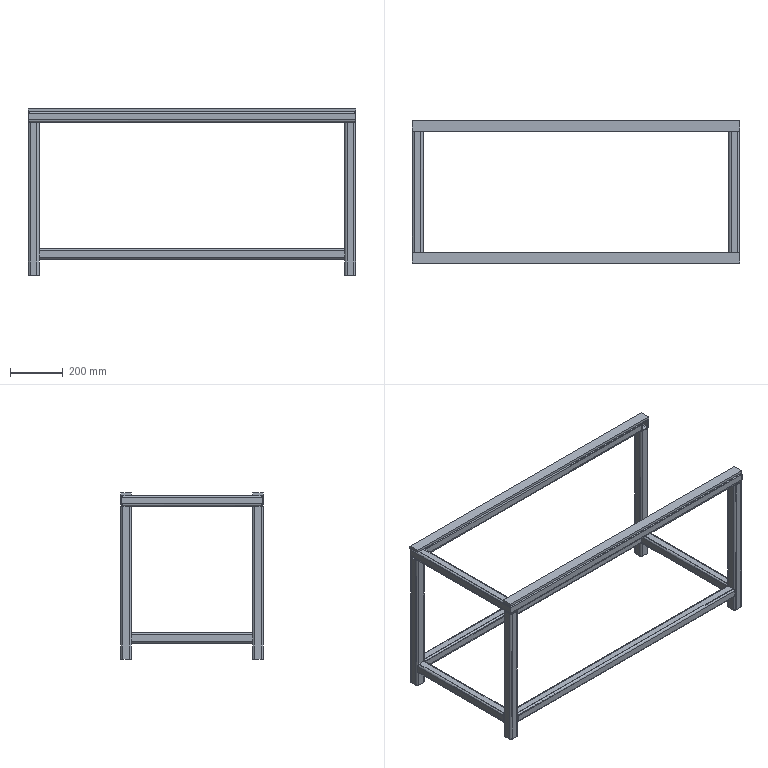Part | SolidWorks | features ICE 2, 3DProfileFeature 1, MirrorSolid 1, WeldMemberFeat 1, WeldmentFeature 1 | 15 solids | 244 faces | box 1240 x 540 x 630 mm | volume 5537770 mm3 | plane 140 | cylinder 104 | commonest cylinder face diameters 8 x52 16 x52